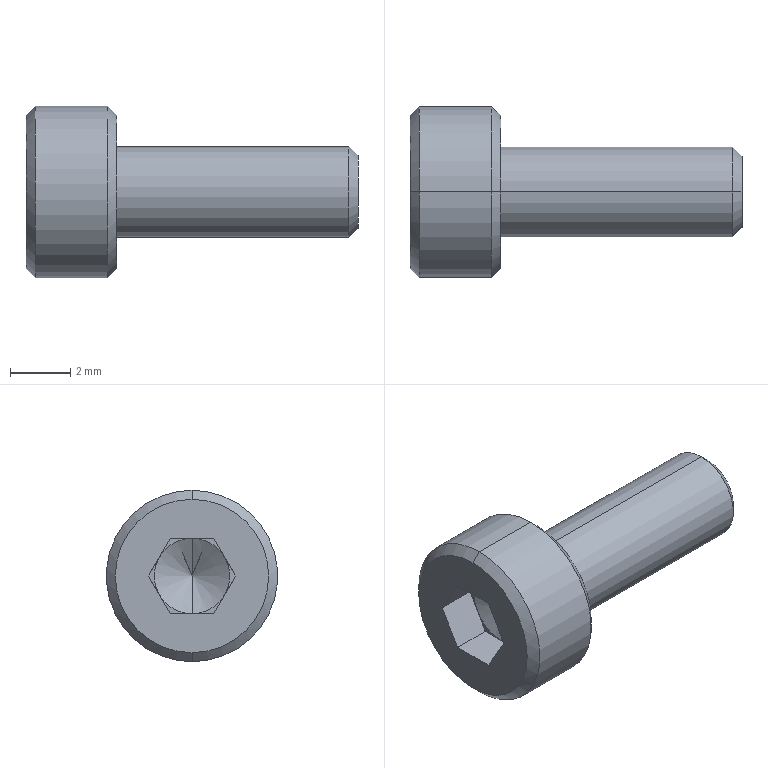Part | STEP file | Hex socket screw Dongming full thread M3-8 A2-70-1 | 1 solid | 27 faces | box 11 x 5.68 x 5.68 mm | volume 122.403 mm3 | plane 15 | cone 8 | cylinder 4 | commonest cylinder face diameters 3 x2 5.68 x2
STEP:
#1=CARTESIAN_POINT('',(11.,0.,-1.2));
#2=VERTEX_POINT('',#1);
#3=CARTESIAN_POINT('',(11.,0.,1.2));
#4=VERTEX_POINT('',#3);
#5=CARTESIAN_POINT('',(11.,0.,0.));
#6=DIRECTION('',(1.,0.,0.));
#7=DIRECTION('',(0.,0.,-1.));
#8=AXIS2_PLACEMENT_3D('',#5,#6,#7);
#9=CIRCLE('',#8,1.2);
#10=EDGE_CURVE('',#2,#4,#9,.T.);
#11=ORIENTED_EDGE('',*,*,#10,.F.);
#12=CARTESIAN_POINT('',(10.7,0.,-1.5));
#13=VERTEX_POINT('',#12);
#14=CARTESIAN_POINT('',(11.,0.,-1.2));
#15=DIRECTION('',(-0.7071,0.,-0.7071));
#16=VECTOR('',#15,1000.);
#17=LINE('',#14,#16);
#18=EDGE_CURVE('',#2,#13,#17,.T.);
#19=ORIENTED_EDGE('',*,*,#18,.T.);
#20=CARTESIAN_POINT('',(10.7,0.,1.5));
#21=VERTEX_POINT('',#20);
#22=CARTESIAN_POINT('',(10.7,0.,0.));
#23=DIRECTION('',(-1.,0.,0.));
#24=DIRECTION('',(0.,0.,-1.));
#25=AXIS2_PLACEMENT_3D('',#22,#23,#24);
#26=CIRCLE('',#25,1.5);
#27=EDGE_CURVE('',#21,#13,#26,.T.);
#28=ORIENTED_EDGE('',*,*,#27,.F.);
#29=CARTESIAN_POINT('',(11.,0.,1.2));
#30=DIRECTION('',(-0.7071,0.,0.7071));
#31=VECTOR('',#30,1000.);
#32=LINE('',#29,#31);
#33=EDGE_CURVE('',#4,#21,#32,.T.);
#34=ORIENTED_EDGE('',*,*,#33,.F.);
#35=EDGE_LOOP('',(#11,#19,#28,#34));
#36=FACE_OUTER_BOUND('',#35,.T.);
#37=CARTESIAN_POINT('',(11.,0.,0.));
#38=DIRECTION('',(-1.,0.,0.));
#39=DIRECTION('',(0.,0.,1.));
#40=AXIS2_PLACEMENT_3D('',#37,#38,#39);
#41=CONICAL_SURFACE('',#40,1.2,0.7854);
#42=ADVANCED_FACE('',(#36),#41,.T.);
#43=CARTESIAN_POINT('',(3.,0.,-2.54));
#44=VERTEX_POINT('',#43);
#45=CARTESIAN_POINT('',(3.,0.,2.54));
#46=VERTEX_POINT('',#45);
#47=CARTESIAN_POINT('',(3.,0.,0.));
#48=DIRECTION('',(1.,0.,0.));
#49=DIRECTION('',(0.,0.,-1.));
#50=AXIS2_PLACEMENT_3D('',#47,#48,#49);
#51=CIRCLE('',#50,2.54);
#52=EDGE_CURVE('',#44,#46,#51,.T.);
#53=ORIENTED_EDGE('',*,*,#52,.F.);
#54=CARTESIAN_POINT('',(2.7,0.,-2.84));
#55=VERTEX_POINT('',#54);
#56=CARTESIAN_POINT('',(3.,0.,-2.54));
#57=DIRECTION('',(-0.7071,0.,-0.7071));
#58=VECTOR('',#57,1000.);
#59=LINE('',#56,#58);
#60=EDGE_CURVE('',#44,#55,#59,.T.);
#61=ORIENTED_EDGE('',*,*,#60,.T.);
#62=CARTESIAN_POINT('',(2.7,0.,2.84));
#63=VERTEX_POINT('',#62);
#64=CARTESIAN_POINT('',(2.7,0.,0.));
#65=DIRECTION('',(-1.,0.,0.));
#66=DIRECTION('',(0.,0.,-1.));
#67=AXIS2_PLACEMENT_3D('',#64,#65,#66);
#68=CIRCLE('',#67,2.84);
#69=EDGE_CURVE('',#63,#55,#68,.T.);
#70=ORIENTED_EDGE('',*,*,#69,.F.);
#71=CARTESIAN_POINT('',(3.,0.,2.54));
#72=DIRECTION('',(-0.7071,0.,0.7071));
#73=VECTOR('',#72,1000.);
#74=LINE('',#71,#73);
#75=EDGE_CURVE('',#46,#63,#74,.T.);
#76=ORIENTED_EDGE('',*,*,#75,.F.);
#77=EDGE_LOOP('',(#53,#61,#70,#76));
#78=FACE_OUTER_BOUND('',#77,.T.);
#79=CARTESIAN_POINT('',(3.,0.,0.));
#80=DIRECTION('',(-1.,0.,0.));
#81=DIRECTION('',(0.,0.,1.));
#82=AXIS2_PLACEMENT_3D('',#79,#80,#81);
#83=CONICAL_SURFACE('',#82,2.54,0.7854);
#84=ADVANCED_FACE('',(#78),#83,.T.);
#85=CARTESIAN_POINT('',(0.,0.,2.54));
#86=VERTEX_POINT('',#85);
#87=CARTESIAN_POINT('',(0.,0.,-2.54));
#88=VERTEX_POINT('',#87);
#89=CARTESIAN_POINT('',(0.,0.,0.));
#90=DIRECTION('',(-1.,0.,0.));
#91=DIRECTION('',(0.,0.,-1.));
#92=AXIS2_PLACEMENT_3D('',#89,#90,#91);
#93=CIRCLE('',#92,2.54);
#94=EDGE_CURVE('',#86,#88,#93,.T.);
#95=ORIENTED_EDGE('',*,*,#94,.F.);
#96=CARTESIAN_POINT('',(0.3,0.,2.84));
#97=VERTEX_POINT('',#96);
#98=CARTESIAN_POINT('',(0.3,0.,2.84));
#99=DIRECTION('',(0.7071,0.,0.7071));
#100=VECTOR('',#99,1000.);
#101=LINE('',#98,#100);
#102=EDGE_CURVE('',#86,#97,#101,.T.);
#103=ORIENTED_EDGE('',*,*,#102,.T.);
#104=CARTESIAN_POINT('',(0.3,0.,-2.84));
#105=VERTEX_POINT('',#104);
#106=CARTESIAN_POINT('',(0.3,0.,0.));
#107=DIRECTION('',(1.,0.,0.));
#108=DIRECTION('',(0.,0.,-1.));
#109=AXIS2_PLACEMENT_3D('',#106,#107,#108);
#110=CIRCLE('',#109,2.84);
#111=EDGE_CURVE('',#105,#97,#110,.T.);
#112=ORIENTED_EDGE('',*,*,#111,.F.);
#113=CARTESIAN_POINT('',(0.3,0.,-2.84));
#114=DIRECTION('',(0.7071,0.,-0.7071));
#115=VECTOR('',#114,1000.);
#116=LINE('',#113,#115);
#117=EDGE_CURVE('',#88,#105,#116,.T.);
#118=ORIENTED_EDGE('',*,*,#117,.F.);
#119=EDGE_LOOP('',(#95,#103,#112,#118));
#120=FACE_OUTER_BOUND('',#119,.T.);
#121=CARTESIAN_POINT('',(0.3,0.,0.));
#122=DIRECTION('',(1.,0.,0.));
#123=DIRECTION('',(0.,0.,-1.));
#124=AXIS2_PLACEMENT_3D('',#121,#122,#123);
#125=CONICAL_SURFACE('',#124,2.84,0.7854);
#126=ADVANCED_FACE('',(#120),#125,.T.);
#127=CARTESIAN_POINT('',(2.022,0.,0.));
#128=VERTEX_POINT('',#127);
#129=CARTESIAN_POINT('',(1.3,0.,1.25));
#130=VERTEX_POINT('',#129);
#131=CARTESIAN_POINT('',(2.022,0.,0.));
#132=DIRECTION('',(-0.5,0.,0.866));
#133=VECTOR('',#132,1000.);
#134=LINE('',#131,#133);
#135=EDGE_CURVE('',#128,#130,#134,.T.);
#136=ORIENTED_EDGE('',*,*,#135,.F.);
#137=CARTESIAN_POINT('',(1.3,0.,-1.25));
#138=VERTEX_POINT('',#137);
#139=CARTESIAN_POINT('',(2.022,0.,0.));
#140=DIRECTION('',(-0.5,0.,-0.866));
#141=VECTOR('',#140,1000.);
#142=LINE('',#139,#141);
#143=EDGE_CURVE('',#128,#138,#142,.T.);
#144=ORIENTED_EDGE('',*,*,#143,.T.);
#145=CARTESIAN_POINT('',(1.3,-1.083,-0.625));
#146=VERTEX_POINT('',#145);
#147=CARTESIAN_POINT('',(1.3,0.,0.));
#148=DIRECTION('',(-1.,0.,0.));
#149=DIRECTION('',(0.,0.,1.));
#150=AXIS2_PLACEMENT_3D('',#147,#148,#149);
#151=CIRCLE('',#150,1.25);
#152=EDGE_CURVE('',#138,#146,#151,.T.);
#153=ORIENTED_EDGE('',*,*,#152,.T.);
#154=CARTESIAN_POINT('',(1.3,-1.083,0.625));
#155=VERTEX_POINT('',#154);
#156=CARTESIAN_POINT('',(1.3,0.,0.));
#157=DIRECTION('',(-1.,0.,0.));
#158=DIRECTION('',(0.,0.,1.));
#159=AXIS2_PLACEMENT_3D('',#156,#157,#158);
#160=CIRCLE('',#159,1.25);
#161=EDGE_CURVE('',#146,#155,#160,.T.);
#162=ORIENTED_EDGE('',*,*,#161,.T.);
#163=CARTESIAN_POINT('',(1.3,0.,0.));
#164=DIRECTION('',(-1.,0.,0.));
#165=DIRECTION('',(0.,0.,1.));
#166=AXIS2_PLACEMENT_3D('',#163,#164,#165);
#167=CIRCLE('',#166,1.25);
#168=EDGE_CURVE('',#155,#130,#167,.T.);
#169=ORIENTED_EDGE('',*,*,#168,.T.);
#170=EDGE_LOOP('',(#136,#144,#153,#162,#169));
#171=FACE_OUTER_BOUND('',#170,.T.);
#172=CARTESIAN_POINT('',(-997.978,0.,0.));
#173=DIRECTION('',(-1.,0.,0.));
#174=DIRECTION('',(0.,0.,1.));
#175=AXIS2_PLACEMENT_3D('',#172,#173,#174);
#176=CONICAL_SURFACE('',#175,1732.051,1.047);
#177=ADVANCED_FACE('',(#171),#176,.F.);
#178=ORIENTED_EDGE('',*,*,#27,.T.);
#179=CARTESIAN_POINT('',(3.,0.,-1.5));
#180=VERTEX_POINT('',#179);
#181=CARTESIAN_POINT('',(11.,0.,-1.5));
#182=DIRECTION('',(-1.,0.,0.));
#183=VECTOR('',#182,1000.);
#184=LINE('',#181,#183);
#185=EDGE_CURVE('',#13,#180,#184,.T.);
#186=ORIENTED_EDGE('',*,*,#185,.T.);
#187=CARTESIAN_POINT('',(3.,0.,1.5));
#188=VERTEX_POINT('',#187);
#189=CARTESIAN_POINT('',(3.,0.,0.));
#190=DIRECTION('',(1.,0.,0.));
#191=DIRECTION('',(0.,0.,-1.));
#192=AXIS2_PLACEMENT_3D('',#189,#190,#191);
#193=CIRCLE('',#192,1.5);
#194=EDGE_CURVE('',#180,#188,#193,.T.);
#195=ORIENTED_EDGE('',*,*,#194,.T.);
#196=CARTESIAN_POINT('',(11.,0.,1.5));
#197=DIRECTION('',(-1.,0.,0.));
#198=VECTOR('',#197,1000.);
#199=LINE('',#196,#198);
#200=EDGE_CURVE('',#21,#188,#199,.T.);
#201=ORIENTED_EDGE('',*,*,#200,.F.);
#202=EDGE_LOOP('',(#178,#186,#195,#201));
#203=FACE_OUTER_BOUND('',#202,.T.);
#204=CARTESIAN_POINT('',(11.,0.,0.));
#205=DIRECTION('',(-1.,0.,0.));
#206=DIRECTION('',(0.,0.,1.));
#207=AXIS2_PLACEMENT_3D('',#204,#205,#206);
#208=CYLINDRICAL_SURFACE('',#207,1.5);
#209=ADVANCED_FACE('',(#203),#208,.T.);
#210=ORIENTED_EDGE('',*,*,#69,.T.);
#211=CARTESIAN_POINT('',(3.,0.,-2.84));
#212=DIRECTION('',(-1.,0.,0.));
#213=VECTOR('',#212,1000.);
#214=LINE('',#211,#213);
#215=EDGE_CURVE('',#55,#105,#214,.T.);
#216=ORIENTED_EDGE('',*,*,#215,.T.);
#217=ORIENTED_EDGE('',*,*,#111,.T.);
#218=CARTESIAN_POINT('',(3.,0.,2.84));
#219=DIRECTION('',(-1.,0.,0.));
#220=VECTOR('',#219,1000.);
#221=LINE('',#218,#220);
#222=EDGE_CURVE('',#63,#97,#221,.T.);
#223=ORIENTED_EDGE('',*,*,#222,.F.);
#224=EDGE_LOOP('',(#210,#216,#217,#223));
#225=FACE_OUTER_BOUND('',#224,.T.);
#226=CARTESIAN_POINT('',(3.,0.,0.));
#227=DIRECTION('',(-1.,0.,0.));
#228=DIRECTION('',(0.,0.,1.));
#229=AXIS2_PLACEMENT_3D('',#226,#227,#228);
#230=CYLINDRICAL_SURFACE('',#229,2.84);
#231=ADVANCED_FACE('',(#225),#230,.T.);
#232=CARTESIAN_POINT('',(1.3,1.083,0.625));
#233=VERTEX_POINT('',#232);
#234=CARTESIAN_POINT('',(1.3,0.,0.));
#235=DIRECTION('',(-1.,0.,0.));
#236=DIRECTION('',(0.,0.,1.));
#237=AXIS2_PLACEMENT_3D('',#234,#235,#236);
#238=CIRCLE('',#237,1.25);
#239=EDGE_CURVE('',#130,#233,#238,.T.);
#240=ORIENTED_EDGE('',*,*,#239,.F.);
#241=CARTESIAN_POINT('',(1.3,0.7217,1.25));
#242=VERTEX_POINT('',#241);
#243=CARTESIAN_POINT('',(1.3,-0.7217,1.25));
#244=DIRECTION('',(0.,1.,0.));
#245=VECTOR('',#244,1000.);
#246=LINE('',#243,#245);
#247=EDGE_CURVE('',#130,#242,#246,.T.);
#248=ORIENTED_EDGE('',*,*,#247,.T.);
#249=CARTESIAN_POINT('',(1.3,0.7217,1.25));
#250=DIRECTION('',(0.,0.5,-0.866));
#251=VECTOR('',#250,1000.);
#252=LINE('',#249,#251);
#253=EDGE_CURVE('',#242,#233,#252,.T.);
#254=ORIENTED_EDGE('',*,*,#253,.T.);
#255=EDGE_LOOP('',(#240,#248,#254));
#256=FACE_OUTER_BOUND('',#255,.T.);
#257=CARTESIAN_POINT('',(1.3,0.,0.));
#258=DIRECTION('',(-1.,0.,0.));
#259=DIRECTION('',(0.,0.,1.));
#260=AXIS2_PLACEMENT_3D('',#257,#258,#259);
#261=PLANE('',#260);
#262=ADVANCED_FACE('',(#256),#261,.T.);
#263=CARTESIAN_POINT('',(1.3,1.083,-0.625));
#264=VERTEX_POINT('',#263);
#265=CARTESIAN_POINT('',(1.3,0.,0.));
#266=DIRECTION('',(-1.,0.,0.));
#267=DIRECTION('',(0.,0.,1.));
#268=AXIS2_PLACEMENT_3D('',#265,#266,#267);
#269=CIRCLE('',#268,1.25);
#270=EDGE_CURVE('',#233,#264,#269,.T.);
#271=ORIENTED_EDGE('',*,*,#270,.F.);
#272=CARTESIAN_POINT('',(1.3,1.443,0.));
#273=VERTEX_POINT('',#272);
#274=CARTESIAN_POINT('',(1.3,0.7217,1.25));
#275=DIRECTION('',(0.,0.5,-0.866));
#276=VECTOR('',#275,1000.);
#277=LINE('',#274,#276);
#278=EDGE_CURVE('',#233,#273,#277,.T.);
#279=ORIENTED_EDGE('',*,*,#278,.T.);
#280=CARTESIAN_POINT('',(1.3,1.443,0.));
#281=DIRECTION('',(0.,-0.5,-0.866));
#282=VECTOR('',#281,1000.);
#283=LINE('',#280,#282);
#284=EDGE_CURVE('',#273,#264,#283,.T.);
#285=ORIENTED_EDGE('',*,*,#284,.T.);
#286=EDGE_LOOP('',(#271,#279,#285));
#287=FACE_OUTER_BOUND('',#286,.T.);
#288=CARTESIAN_POINT('',(1.3,0.,0.));
#289=DIRECTION('',(-1.,0.,0.));
#290=DIRECTION('',(0.,0.,1.));
#291=AXIS2_PLACEMENT_3D('',#288,#289,#290);
#292=PLANE('',#291);
#293=ADVANCED_FACE('',(#287),#292,.T.);
#294=CARTESIAN_POINT('',(1.3,0.,0.));
#295=DIRECTION('',(-1.,0.,0.));
#296=DIRECTION('',(0.,0.,1.));
#297=AXIS2_PLACEMENT_3D('',#294,#295,#296);
#298=CIRCLE('',#297,1.25);
#299=EDGE_CURVE('',#264,#138,#298,.T.);
#300=ORIENTED_EDGE('',*,*,#299,.F.);
#301=CARTESIAN_POINT('',(1.3,0.7217,-1.25));
#302=VERTEX_POINT('',#301);
#303=CARTESIAN_POINT('',(1.3,1.443,0.));
#304=DIRECTION('',(0.,-0.5,-0.866));
#305=VECTOR('',#304,1000.);
#306=LINE('',#303,#305);
#307=EDGE_CURVE('',#264,#302,#306,.T.);
#308=ORIENTED_EDGE('',*,*,#307,.T.);
#309=CARTESIAN_POINT('',(1.3,0.7217,-1.25));
#310=DIRECTION('',(0.,-1.,0.));
#311=VECTOR('',#310,1000.);
#312=LINE('',#309,#311);
#313=EDGE_CURVE('',#302,#138,#312,.T.);
#314=ORIENTED_EDGE('',*,*,#313,.T.);
#315=EDGE_LOOP('',(#300,#308,#314));
#316=FACE_OUTER_BOUND('',#315,.T.);
#317=CARTESIAN_POINT('',(1.3,0.,0.));
#318=DIRECTION('',(-1.,0.,0.));
#319=DIRECTION('',(0.,0.,1.));
#320=AXIS2_PLACEMENT_3D('',#317,#318,#319);
#321=PLANE('',#320);
#322=ADVANCED_FACE('',(#316),#321,.T.);
#323=ORIENTED_EDGE('',*,*,#152,.F.);
#324=CARTESIAN_POINT('',(1.3,-0.7217,-1.25));
#325=VERTEX_POINT('',#324);
#326=CARTESIAN_POINT('',(1.3,0.7217,-1.25));
#327=DIRECTION('',(0.,-1.,0.));
#328=VECTOR('',#327,1000.);
#329=LINE('',#326,#328);
#330=EDGE_CURVE('',#138,#325,#329,.T.);
#331=ORIENTED_EDGE('',*,*,#330,.T.);
#332=CARTESIAN_POINT('',(1.3,-0.7217,-1.25));
#333=DIRECTION('',(0.,-0.5,0.866));
#334=VECTOR('',#333,1000.);
#335=LINE('',#332,#334);
#336=EDGE_CURVE('',#325,#146,#335,.T.);
#337=ORIENTED_EDGE('',*,*,#336,.T.);
#338=EDGE_LOOP('',(#323,#331,#337));
#339=FACE_OUTER_BOUND('',#338,.T.);
#340=CARTESIAN_POINT('',(1.3,0.,0.));
#341=DIRECTION('',(-1.,0.,0.));
#342=DIRECTION('',(0.,0.,1.));
#343=AXIS2_PLACEMENT_3D('',#340,#341,#342);
#344=PLANE('',#343);
#345=ADVANCED_FACE('',(#339),#344,.T.);
#346=ORIENTED_EDGE('',*,*,#161,.F.);
#347=CARTESIAN_POINT('',(1.3,-1.443,0.));
#348=VERTEX_POINT('',#347);
#349=CARTESIAN_POINT('',(1.3,-0.7217,-1.25));
#350=DIRECTION('',(0.,-0.5,0.866));
#351=VECTOR('',#350,1000.);
#352=LINE('',#349,#351);
#353=EDGE_CURVE('',#146,#348,#352,.T.);
#354=ORIENTED_EDGE('',*,*,#353,.T.);
#355=CARTESIAN_POINT('',(1.3,-1.443,0.));
#356=DIRECTION('',(0.,0.5,0.866));
#357=VECTOR('',#356,1000.);
#358=LINE('',#355,#357);
#359=EDGE_CURVE('',#348,#155,#358,.T.);
#360=ORIENTED_EDGE('',*,*,#359,.T.);
#361=EDGE_LOOP('',(#346,#354,#360));
#362=FACE_OUTER_BOUND('',#361,.T.);
#363=CARTESIAN_POINT('',(1.3,0.,0.));
#364=DIRECTION('',(-1.,0.,0.));
#365=DIRECTION('',(0.,0.,1.));
#366=AXIS2_PLACEMENT_3D('',#363,#364,#365);
#367=PLANE('',#366);
#368=ADVANCED_FACE('',(#362),#367,.T.);
#369=ORIENTED_EDGE('',*,*,#215,.F.);
#370=CARTESIAN_POINT('',(2.7,0.,0.));
#371=DIRECTION('',(-1.,0.,0.));
#372=DIRECTION('',(0.,0.,-1.));
#373=AXIS2_PLACEMENT_3D('',#370,#371,#372);
#374=CIRCLE('',#373,2.84);
#375=EDGE_CURVE('',#55,#63,#374,.T.);
#376=ORIENTED_EDGE('',*,*,#375,.T.);
#377=ORIENTED_EDGE('',*,*,#222,.T.);
#378=CARTESIAN_POINT('',(0.3,0.,0.));
#379=DIRECTION('',(1.,0.,0.));
#380=DIRECTION('',(0.,0.,-1.));
#381=AXIS2_PLACEMENT_3D('',#378,#379,#380);
#382=CIRCLE('',#381,2.84);
#383=EDGE_CURVE('',#97,#105,#382,.T.);
#384=ORIENTED_EDGE('',*,*,#383,.T.);
#385=EDGE_LOOP('',(#369,#376,#377,#384));
#386=FACE_OUTER_BOUND('',#385,.T.);
#387=CARTESIAN_POINT('',(3.,0.,0.));
#388=DIRECTION('',(-1.,0.,0.));
#389=DIRECTION('',(0.,0.,1.));
#390=AXIS2_PLACEMENT_3D('',#387,#388,#389);
#391=CYLINDRICAL_SURFACE('',#390,2.84);
#392=ADVANCED_FACE('',(#386),#391,.T.);
#393=CARTESIAN_POINT('',(3.,0.,0.));
#394=DIRECTION('',(1.,0.,0.));
#395=DIRECTION('',(0.,0.,-1.));
#396=AXIS2_PLACEMENT_3D('',#393,#394,#395);
#397=CIRCLE('',#396,2.54);
#398=EDGE_CURVE('',#46,#44,#397,.T.);
#399=ORIENTED_EDGE('',*,*,#398,.T.);
#400=ORIENTED_EDGE('',*,*,#52,.T.);
#401=EDGE_LOOP('',(#399,#400));
#402=FACE_OUTER_BOUND('',#401,.T.);
#403=CARTESIAN_POINT('',(3.,0.,0.));
#404=DIRECTION('',(1.,0.,0.));
#405=DIRECTION('',(0.,0.,-1.));
#406=AXIS2_PLACEMENT_3D('',#403,#404,#405);
#407=CIRCLE('',#406,1.5);
#408=EDGE_CURVE('',#188,#180,#407,.T.);
#409=ORIENTED_EDGE('',*,*,#408,.F.);
#410=ORIENTED_EDGE('',*,*,#194,.F.);
#411=EDGE_LOOP('',(#409,#410));
#412=FACE_BOUND('',#411,.T.);
#413=CARTESIAN_POINT('',(3.,0.,0.));
#414=DIRECTION('',(1.,0.,0.));
#415=DIRECTION('',(0.,0.,-1.));
#416=AXIS2_PLACEMENT_3D('',#413,#414,#415);
#417=PLANE('',#416);
#418=ADVANCED_FACE('',(#402,#412),#417,.T.);
#419=CARTESIAN_POINT('',(0.,0.,0.));
#420=DIRECTION('',(-1.,0.,0.));
#421=DIRECTION('',(0.,0.,-1.));
#422=AXIS2_PLACEMENT_3D('',#419,#420,#421);
#423=CIRCLE('',#422,2.54);
#424=EDGE_CURVE('',#88,#86,#423,.T.);
#425=ORIENTED_EDGE('',*,*,#424,.T.);
#426=ORIENTED_EDGE('',*,*,#94,.T.);
#427=EDGE_LOOP('',(#425,#426));
#428=FACE_OUTER_BOUND('',#427,.T.);
#429=CARTESIAN_POINT('',(0.,1.443,0.));
#430=VERTEX_POINT('',#429);
#431=CARTESIAN_POINT('',(0.,0.7217,-1.25));
#432=VERTEX_POINT('',#431);
#433=CARTESIAN_POINT('',(0.,1.443,0.));
#434=DIRECTION('',(0.,-0.5,-0.866));
#435=VECTOR('',#434,1000.);
#436=LINE('',#433,#435);
#437=EDGE_CURVE('',#430,#432,#436,.T.);
#438=ORIENTED_EDGE('',*,*,#437,.F.);
#439=CARTESIAN_POINT('',(0.,0.7217,1.25));
#440=VERTEX_POINT('',#439);
#441=CARTESIAN_POINT('',(0.,0.7217,1.25));
#442=DIRECTION('',(0.,0.5,-0.866));
#443=VECTOR('',#442,1000.);
#444=LINE('',#441,#443);
#445=EDGE_CURVE('',#440,#430,#444,.T.);
#446=ORIENTED_EDGE('',*,*,#445,.F.);
#447=CARTESIAN_POINT('',(0.,-0.7217,1.25));
#448=VERTEX_POINT('',#447);
#449=CARTESIAN_POINT('',(0.,-0.7217,1.25));
#450=DIRECTION('',(0.,1.,0.));
#451=VECTOR('',#450,1000.);
#452=LINE('',#449,#451);
#453=EDGE_CURVE('',#448,#440,#452,.T.);
#454=ORIENTED_EDGE('',*,*,#453,.F.);
#455=CARTESIAN_POINT('',(0.,-1.443,0.));
#456=VERTEX_POINT('',#455);
#457=CARTESIAN_POINT('',(0.,-1.443,0.));
#458=DIRECTION('',(0.,0.5,0.866));
#459=VECTOR('',#458,1000.);
#460=LINE('',#457,#459);
#461=EDGE_CURVE('',#456,#448,#460,.T.);
#462=ORIENTED_EDGE('',*,*,#461,.F.);
#463=CARTESIAN_POINT('',(0.,-0.7217,-1.25));
#464=VERTEX_POINT('',#463);
#465=CARTESIAN_POINT('',(0.,-0.7217,-1.25));
#466=DIRECTION('',(0.,-0.5,0.866));
#467=VECTOR('',#466,1000.);
#468=LINE('',#465,#467);
#469=EDGE_CURVE('',#464,#456,#468,.T.);
#470=ORIENTED_EDGE('',*,*,#469,.F.);
#471=CARTESIAN_POINT('',(0.,0.7217,-1.25));
#472=DIRECTION('',(0.,-1.,0.));
#473=VECTOR('',#472,1000.);
#474=LINE('',#471,#473);
#475=EDGE_CURVE('',#432,#464,#474,.T.);
#476=ORIENTED_EDGE('',*,*,#475,.F.);
#477=EDGE_LOOP('',(#438,#446,#454,#462,#470,#476));
#478=FACE_BOUND('',#477,.T.);
#479=CARTESIAN_POINT('',(0.,0.,0.));
#480=DIRECTION('',(1.,0.,0.));
#481=DIRECTION('',(0.,0.,-1.));
#482=AXIS2_PLACEMENT_3D('',#479,#480,#481);
#483=PLANE('',#482);
#484=ADVANCED_FACE('',(#428,#478),#483,.F.);
#485=ORIENTED_EDGE('',*,*,#185,.F.);
#486=CARTESIAN_POINT('',(10.7,0.,0.));
#487=DIRECTION('',(-1.,0.,0.));
#488=DIRECTION('',(0.,0.,-1.));
#489=AXIS2_PLACEMENT_3D('',#486,#487,#488);
#490=CIRCLE('',#489,1.5);
#491=EDGE_CURVE('',#13,#21,#490,.T.);
#492=ORIENTED_EDGE('',*,*,#491,.T.);
#493=ORIENTED_EDGE('',*,*,#200,.T.);
#494=ORIENTED_EDGE('',*,*,#408,.T.);
#495=EDGE_LOOP('',(#485,#492,#493,#494));
#496=FACE_OUTER_BOUND('',#495,.T.);
#497=CARTESIAN_POINT('',(11.,0.,0.));
#498=DIRECTION('',(-1.,0.,0.));
#499=DIRECTION('',(0.,0.,1.));
#500=AXIS2_PLACEMENT_3D('',#497,#498,#499);
#501=CYLINDRICAL_SURFACE('',#500,1.5);
#502=ADVANCED_FACE('',(#496),#501,.T.);
#503=CARTESIAN_POINT('',(11.,0.,0.));
#504=DIRECTION('',(1.,0.,0.));
#505=DIRECTION('',(0.,0.,-1.));
#506=AXIS2_PLACEMENT_3D('',#503,#504,#505);
#507=CIRCLE('',#506,1.2);
#508=EDGE_CURVE('',#4,#2,#507,.T.);
#509=ORIENTED_EDGE('',*,*,#508,.T.);
#510=ORIENTED_EDGE('',*,*,#10,.T.);
#511=EDGE_LOOP('',(#509,#510));
#512=FACE_OUTER_BOUND('',#511,.T.);
#513=CARTESIAN_POINT('',(11.,0.,0.));
#514=DIRECTION('',(1.,0.,0.));
#515=DIRECTION('',(0.,0.,-1.));
#516=AXIS2_PLACEMENT_3D('',#513,#514,#515);
#517=PLANE('',#516);
#518=ADVANCED_FACE('',(#512),#517,.T.);
#519=ORIENTED_EDGE('',*,*,#445,.T.);
#520=CARTESIAN_POINT('',(1.3,1.443,0.));
#521=DIRECTION('',(-1.,0.,0.));
#522=VECTOR('',#521,1000.);
#523=LINE('',#520,#522);
#524=EDGE_CURVE('',#273,#430,#523,.T.);
#525=ORIENTED_EDGE('',*,*,#524,.F.);
#526=ORIENTED_EDGE('',*,*,#278,.F.);
#527=ORIENTED_EDGE('',*,*,#253,.F.);
#528=CARTESIAN_POINT('',(1.3,0.7217,1.25));
#529=DIRECTION('',(-1.,0.,0.));
#530=VECTOR('',#529,1000.);
#531=LINE('',#528,#530);
#532=EDGE_CURVE('',#242,#440,#531,.T.);
#533=ORIENTED_EDGE('',*,*,#532,.T.);
#534=EDGE_LOOP('',(#519,#525,#526,#527,#533));
#535=FACE_OUTER_BOUND('',#534,.T.);
#536=CARTESIAN_POINT('',(1.3,0.7217,1.25));
#537=DIRECTION('',(0.,0.866,0.5));
#538=DIRECTION('',(0.,-0.5,0.866));
#539=AXIS2_PLACEMENT_3D('',#536,#537,#538);
#540=PLANE('',#539);
#541=ADVANCED_FACE('',(#535),#540,.F.);
#542=ORIENTED_EDGE('',*,*,#453,.T.);
#543=ORIENTED_EDGE('',*,*,#532,.F.);
#544=ORIENTED_EDGE('',*,*,#247,.F.);
#545=CARTESIAN_POINT('',(1.3,-0.7217,1.25));
#546=VERTEX_POINT('',#545);
#547=CARTESIAN_POINT('',(1.3,-0.7217,1.25));
#548=DIRECTION('',(0.,1.,0.));
#549=VECTOR('',#548,1000.);
#550=LINE('',#547,#549);
#551=EDGE_CURVE('',#546,#130,#550,.T.);
#552=ORIENTED_EDGE('',*,*,#551,.F.);
#553=CARTESIAN_POINT('',(1.3,-0.7217,1.25));
#554=DIRECTION('',(-1.,0.,0.));
#555=VECTOR('',#554,1000.);
#556=LINE('',#553,#555);
#557=EDGE_CURVE('',#546,#448,#556,.T.);
#558=ORIENTED_EDGE('',*,*,#557,.T.);
#559=EDGE_LOOP('',(#542,#543,#544,#552,#558));
#560=FACE_OUTER_BOUND('',#559,.T.);
#561=CARTESIAN_POINT('',(1.3,-0.7217,1.25));
#562=DIRECTION('',(0.,0.,1.));
#563=DIRECTION('',(0.,-1.,0.));
#564=AXIS2_PLACEMENT_3D('',#561,#562,#563);
#565=PLANE('',#564);
#566=ADVANCED_FACE('',(#560),#565,.F.);
#567=ORIENTED_EDGE('',*,*,#461,.T.);
#568=ORIENTED_EDGE('',*,*,#557,.F.);
#569=CARTESIAN_POINT('',(1.3,-1.443,0.));
#570=DIRECTION('',(0.,0.5,0.866));
#571=VECTOR('',#570,1000.);
#572=LINE('',#569,#571);
#573=EDGE_CURVE('',#155,#546,#572,.T.);
#574=ORIENTED_EDGE('',*,*,#573,.F.);
#575=ORIENTED_EDGE('',*,*,#359,.F.);
#576=CARTESIAN_POINT('',(1.3,-1.443,0.));
#577=DIRECTION('',(-1.,0.,0.));
#578=VECTOR('',#577,1000.);
#579=LINE('',#576,#578);
#580=EDGE_CURVE('',#348,#456,#579,.T.);
#581=ORIENTED_EDGE('',*,*,#580,.T.);
#582=EDGE_LOOP('',(#567,#568,#574,#575,#581));
#583=FACE_OUTER_BOUND('',#582,.T.);
#584=CARTESIAN_POINT('',(1.3,-1.443,0.));
#585=DIRECTION('',(0.,-0.866,0.5));
#586=DIRECTION('',(0.,-0.5,-0.866));
#587=AXIS2_PLACEMENT_3D('',#584,#585,#586);
#588=PLANE('',#587);
#589=ADVANCED_FACE('',(#583),#588,.F.);
#590=ORIENTED_EDGE('',*,*,#469,.T.);
#591=ORIENTED_EDGE('',*,*,#580,.F.);
#592=ORIENTED_EDGE('',*,*,#353,.F.);
#593=ORIENTED_EDGE('',*,*,#336,.F.);
#594=CARTESIAN_POINT('',(1.3,-0.7217,-1.25));
#595=DIRECTION('',(-1.,0.,0.));
#596=VECTOR('',#595,1000.);
#597=LINE('',#594,#596);
#598=EDGE_CURVE('',#325,#464,#597,.T.);
#599=ORIENTED_EDGE('',*,*,#598,.T.);
#600=EDGE_LOOP('',(#590,#591,#592,#593,#599));
#601=FACE_OUTER_BOUND('',#600,.T.);
#602=CARTESIAN_POINT('',(1.3,-0.7217,-1.25));
#603=DIRECTION('',(0.,-0.866,-0.5));
#604=DIRECTION('',(0.,0.5,-0.866));
#605=AXIS2_PLACEMENT_3D('',#602,#603,#604);
#606=PLANE('',#605);
#607=ADVANCED_FACE('',(#601),#606,.F.);
#608=ORIENTED_EDGE('',*,*,#475,.T.);
#609=ORIENTED_EDGE('',*,*,#598,.F.);
#610=ORIENTED_EDGE('',*,*,#330,.F.);
#611=ORIENTED_EDGE('',*,*,#313,.F.);
#612=CARTESIAN_POINT('',(1.3,0.7217,-1.25));
#613=DIRECTION('',(-1.,0.,0.));
#614=VECTOR('',#613,1000.);
#615=LINE('',#612,#614);
#616=EDGE_CURVE('',#302,#432,#615,.T.);
#617=ORIENTED_EDGE('',*,*,#616,.T.);
#618=EDGE_LOOP('',(#608,#609,#610,#611,#617));
#619=FACE_OUTER_BOUND('',#618,.T.);
#620=CARTESIAN_POINT('',(1.3,0.7217,-1.25));
#621=DIRECTION('',(0.,0.,-1.));
#622=DIRECTION('',(-1.,0.,0.));
#623=AXIS2_PLACEMENT_3D('',#620,#621,#622);
#624=PLANE('',#623);
#625=ADVANCED_FACE('',(#619),#624,.F.);
#626=ORIENTED_EDGE('',*,*,#437,.T.);
#627=ORIENTED_EDGE('',*,*,#616,.F.);
#628=ORIENTED_EDGE('',*,*,#307,.F.);
#629=ORIENTED_EDGE('',*,*,#284,.F.);
#630=ORIENTED_EDGE('',*,*,#524,.T.);
#631=EDGE_LOOP('',(#626,#627,#628,#629,#630));
#632=FACE_OUTER_BOUND('',#631,.T.);
#633=CARTESIAN_POINT('',(1.3,1.443,0.));
#634=DIRECTION('',(0.,0.866,-0.5));
#635=DIRECTION('',(0.,0.5,0.866));
#636=AXIS2_PLACEMENT_3D('',#633,#634,#635);
#637=PLANE('',#636);
#638=ADVANCED_FACE('',(#632),#637,.F.);
#639=ORIENTED_EDGE('',*,*,#168,.F.);
#640=ORIENTED_EDGE('',*,*,#573,.T.);
#641=ORIENTED_EDGE('',*,*,#551,.T.);
#642=EDGE_LOOP('',(#639,#640,#641));
#643=FACE_OUTER_BOUND('',#642,.T.);
#644=CARTESIAN_POINT('',(1.3,0.,0.));
#645=DIRECTION('',(-1.,0.,0.));
#646=DIRECTION('',(0.,0.,1.));
#647=AXIS2_PLACEMENT_3D('',#644,#645,#646);
#648=PLANE('',#647);
#649=ADVANCED_FACE('',(#643),#648,.T.);
#650=ORIENTED_EDGE('',*,*,#143,.F.);
#651=ORIENTED_EDGE('',*,*,#135,.T.);
#652=ORIENTED_EDGE('',*,*,#239,.T.);
#653=ORIENTED_EDGE('',*,*,#270,.T.);
#654=ORIENTED_EDGE('',*,*,#299,.T.);
#655=EDGE_LOOP('',(#650,#651,#652,#653,#654));
#656=FACE_OUTER_BOUND('',#655,.T.);
#657=CARTESIAN_POINT('',(-997.978,0.,0.));
#658=DIRECTION('',(-1.,0.,0.));
#659=DIRECTION('',(0.,0.,1.));
#660=AXIS2_PLACEMENT_3D('',#657,#658,#659);
#661=CONICAL_SURFACE('',#660,1732.051,1.047);
#662=ADVANCED_FACE('',(#656),#661,.F.);
#663=ORIENTED_EDGE('',*,*,#102,.F.);
#664=ORIENTED_EDGE('',*,*,#424,.F.);
#665=ORIENTED_EDGE('',*,*,#117,.T.);
#666=ORIENTED_EDGE('',*,*,#383,.F.);
#667=EDGE_LOOP('',(#663,#664,#665,#666));
#668=FACE_OUTER_BOUND('',#667,.T.);
#669=CARTESIAN_POINT('',(0.3,0.,0.));
#670=DIRECTION('',(1.,0.,0.));
#671=DIRECTION('',(0.,0.,-1.));
#672=AXIS2_PLACEMENT_3D('',#669,#670,#671);
#673=CONICAL_SURFACE('',#672,2.84,0.7854);
#674=ADVANCED_FACE('',(#668),#673,.T.);
#675=ORIENTED_EDGE('',*,*,#60,.F.);
#676=ORIENTED_EDGE('',*,*,#398,.F.);
#677=ORIENTED_EDGE('',*,*,#75,.T.);
#678=ORIENTED_EDGE('',*,*,#375,.F.);
#679=EDGE_LOOP('',(#675,#676,#677,#678));
#680=FACE_OUTER_BOUND('',#679,.T.);
#681=CARTESIAN_POINT('',(3.,0.,0.));
#682=DIRECTION('',(-1.,0.,0.));
#683=DIRECTION('',(0.,0.,1.));
#684=AXIS2_PLACEMENT_3D('',#681,#682,#683);
#685=CONICAL_SURFACE('',#684,2.54,0.7854);
#686=ADVANCED_FACE('',(#680),#685,.T.);
#687=ORIENTED_EDGE('',*,*,#18,.F.);
#688=ORIENTED_EDGE('',*,*,#508,.F.);
#689=ORIENTED_EDGE('',*,*,#33,.T.);
#690=ORIENTED_EDGE('',*,*,#491,.F.);
#691=EDGE_LOOP('',(#687,#688,#689,#690));
#692=FACE_OUTER_BOUND('',#691,.T.);
#693=CARTESIAN_POINT('',(11.,0.,0.));
#694=DIRECTION('',(-1.,0.,0.));
#695=DIRECTION('',(0.,0.,1.));
#696=AXIS2_PLACEMENT_3D('',#693,#694,#695);
#697=CONICAL_SURFACE('',#696,1.2,0.7854);
#698=ADVANCED_FACE('',(#692),#697,.T.);
#699=CLOSED_SHELL('',(#42,#84,#126,#177,#209,#231,#262,#293,#322,#345,#368,#392,#418,#484,#502,#518,#541,#566,#589,#607,#625,#638,#649,#662,#674,#686,#698));
#700=MANIFOLD_SOLID_BREP('',#699);
#701=CARTESIAN_POINT('',(0.,0.,0.));
#702=DIRECTION('',(0.,0.,1.));
#703=DIRECTION('',(1.,0.,0.));
#704=AXIS2_PLACEMENT_3D('',#701,#702,#703);
#705=(LENGTH_UNIT()NAMED_UNIT(*)SI_UNIT(.MILLI.,.METRE.));
#706=UNCERTAINTY_MEASURE_WITH_UNIT(LENGTH_MEASURE(0.00001),#705,'','');
#707=(NAMED_UNIT(*)PLANE_ANGLE_UNIT()SI_UNIT($,.RADIAN.));
#708=(NAMED_UNIT(*)SI_UNIT($,.STERADIAN.)SOLID_ANGLE_UNIT());
#709=(GEOMETRIC_REPRESENTATION_CONTEXT(3)GLOBAL_UNCERTAINTY_ASSIGNED_CONTEXT((#706))GLOBAL_UNIT_ASSIGNED_CONTEXT((#705,#707,#708))REPRESENTATION_CONTEXT('',''));
#710=ADVANCED_BREP_SHAPE_REPRESENTATION('',(#700,#704),#709);